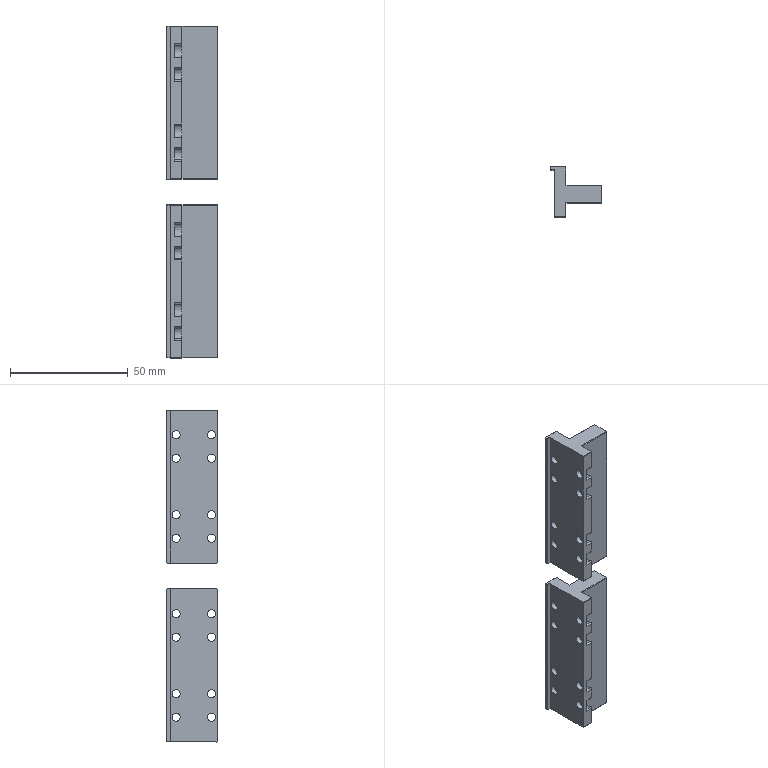CAM job | NX | 3+2 milling, drilling | part box 21.5 x 21.5 x 141 mm | stock box 25 x 25 x 146 mm
Tools:
number,name,description,diameter,corner_radius,flute_length,length,flutes
4,D4,平底铣刀-粗,4.0,0.0,25.0,75.0,2
9,D10,平底铣刀-粗,10.0,0.0,35.0,75.0,2
11,D4-J,平底铣刀-精,4.0,0.0,50.0,75.0,2
10,D10-J,平底铣刀-精,10.0,0.0,35.0,75.0,2
1,D80R0.8飞刀,圆鼻刀-粗,80.0,0.8,50.0,75.0,2
1,D80R0.8飞刀-J,圆鼻刀-精,80.0,0.8,50.0,75.0,2
2,D6倒角刀,倒角刀,6.0,0.0,3.0,25.0,2
21,M4X0.7,丝锥,3.3,0.0,35.0,50.0,2
17,ZT3.5,钻头,3.5,0.0,35.0,50.0,2
13,钻头3.3,Twist Drill 3.3 mm,3.3,0.0,35.0,35.008,2
Operations:
program,operation,operation_type,tool,method,geometry_group,spindle_rpm,surface_speed,feed_per_tooth,feed_cut,feed_plunge,cut_length_mm,path_length_mm,cut_time_min,machine_time_min
B,底壁铣飞面一刀开粗_COPY,VolumeBased25DMillingOperation,D80R0.8飞刀,分层开粗-切深K-步距G,W-B,2800.0,703.696,0.5357,3000.0,100.0,1744.358,3351.438,0.5815,0.7422
B,底壁铣飞面一刀精光_COPY,VolumeBased25DMillingOperation,D80R0.8飞刀-J,侧刃精光-切深K-步距G,W-B,4000.0,1005.28,0.125,1000.0,100.0,248.998,284.998,0.249,0.2526
B,底壁铣分层开粗-中_COPY,VolumeBased25DMillingOperation,D10,分层开粗-切深K-步距G,W-B,8000.0,251.32,0.25,4000.0,100.0,1927.049,1953.884,0.4818,0.4844
B,平面去毛刺6X45L_COPY_1,SurfaceContour,D6倒角刀,爬面_倒角-切深0-步距G,W-B,6500.0,122.519,0.1154,1500.0,100.0,656.729,1320.447,0.4378,0.5042
B,底壁铣精光底面-中_COPY,VolumeBased25DMillingOperation,D10-J,精光步距切深关,W-B,8000.0,251.32,0.0625,1000.0,100.0,776.049,802.649,0.776,0.7787
B,底壁铣精光侧面-中-选底面_COPY,VolumeBased25DMillingOperation,D10-J,侧刃精光-切深K-步距G,W-B,8000.0,251.32,0.0625,1000.0,100.0,160.002,187.602,0.16,0.1628
A,顶面,FaceMilling,D80R0.8飞刀,侧刃精光-切深K-步距G,W-A,4000.0,1005.31,0.125,1000.0,100.0,235.0,271.0,0.235,0.2386
A,外形粗_2,VolumeBased25DMillingOperation,D10,METHOD,W-A,8000.0,251.327,0.3125,5000.0,80.0,11868.472,12065.372,2.374,2.393
A,底壁粗_1,VolumeBased25DMillingOperation,D10,METHOD,W-A,8000.0,251.327,0.3125,5000.0,100.0,8962.764,9641.831,1.793,1.861
A,底壁粗_2,VolumeBased25DMillingOperation,D10,METHOD,W-A,8000.0,251.327,0.3125,5000.0,100.0,8915.44,9594.507,1.783,1.851
A,打点-深0.8,Operation,D6倒角刀,NONE,W-A,8000.0,150.796,0.0312,500.0,90.0,39.6,524.996,0.0792,0.1277
A,沉头孔-钻孔0段,Operation,ZT3.5,NONE,W-A,2800.0,30.788,0.0179,100.0,90.0,144.824,601.282,1.448,1.494
A,盲平孔-M4螺纹底孔,Operation,钻头3.3,NONE,W-A,3000.0,31.102,0.0167,100.0,90.0,84.0,339.099,0.84,0.8655
A,底壁粗_3,VolumeBased25DMillingOperation,D4,METHOD,W-A,6000.0,75.398,0.1,1200.0,100.0,1525.366,2711.528,1.271,1.39
A,铣孔开粗D4_1,CylinderMilling,D4,NONE,W-A,8000.0,100.531,0.075,1200.0,100.0,1192.776,2581.86,0.994,1.133
A,平面去毛刺6X45L_COPY,SurfaceContour,D6倒角刀,爬面_倒角-切深0-步距G,W-A,6500.0,122.519,0.1154,1500.0,100.0,1332.893,2450.445,0.8886,1
A,钻倒角_1,Operation,D6倒角刀,METHOD,W-A,8000.0,150.796,0.0312,500.0,0.0,31.2,244.29,0.0624,0.0837
A,盲平孔-攻牙M4,Operation,M4X0.7,METHOD,W-A,800.0,8.294,0.0004,0.7,90.0,60.0,291.099,85.714,85.737
A,铣孔精光D4_1,CylinderMilling,D4-J,精光步距切深关,W-A,8000.0,100.531,0.0312,500.0,100.0,119.528,819.528,0.2391,0.3091
A,底侧精_5,VolumeBased25DMillingOperation,D4-J,METHOD,W-A,6000.0,113.0,0.2083,1200.0,100.0,184.417,977.182,0.1537,0.233
A,底侧精_3,VolumeBased25DMillingOperation,D10-J,METHOD,W-A,6000.0,113.0,0.2083,1200.0,100.0,323.455,745.245,0.2695,0.3117
A,底侧精_4,VolumeBased25DMillingOperation,D10-J,METHOD,W-A,6000.0,113.0,0.2083,1200.0,100.0,323.455,745.245,0.2695,0.3117
A,外形半精_2,VolumeBased25DMillingOperation,D10-J,METHOD,W-A,8000.0,251.327,0.0625,1000.0,100.0,844.164,1188.578,0.8442,0.8786